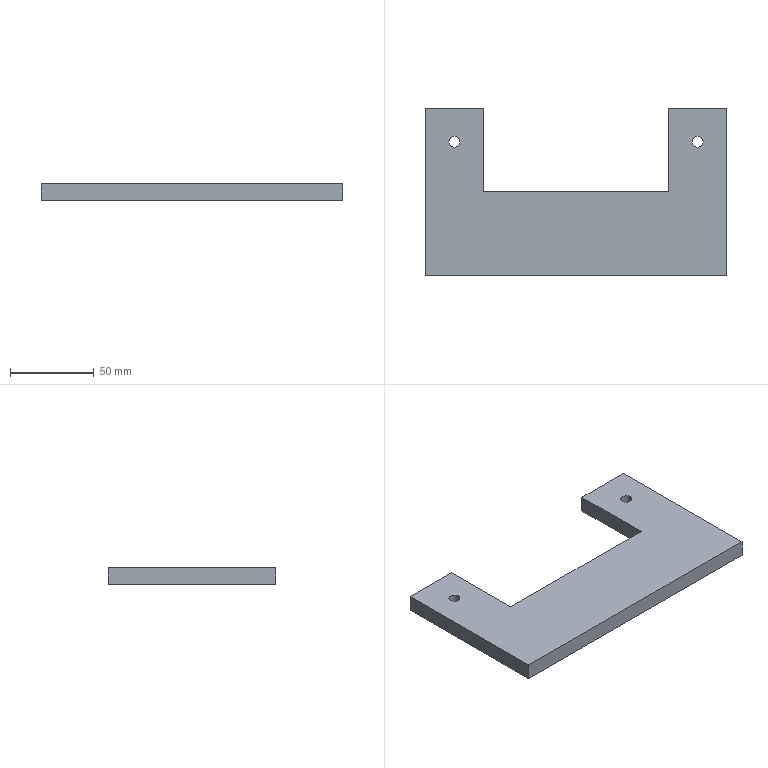Part | SolidWorks | features Extrusion 1, HoleWzd 1, ICE 1 | 1 solid | 14 faces | box 180 x 100 x 10 mm | volume 124316 mm3 | plane 10 | cylinder 4 | commonest cylinder face diameters 6.6 x4
STEP:
#1=CARTESIAN_POINT('',(69.2,30.,10.));
#2=VERTEX_POINT('',#1);
#3=CARTESIAN_POINT('',(75.8,30.,10.));
#4=VERTEX_POINT('',#3);
#5=CARTESIAN_POINT('',(72.5,30.,10.));
#6=DIRECTION('',(0.,0.,1.));
#7=DIRECTION('',(1.,0.,0.));
#8=AXIS2_PLACEMENT_3D('',#5,#6,#7);
#9=CIRCLE('',#8,3.3);
#10=EDGE_CURVE('',#2,#4,#9,.T.);
#11=ORIENTED_EDGE('',*,*,#10,.T.);
#12=CARTESIAN_POINT('',(75.8,30.,0.));
#13=VERTEX_POINT('',#12);
#14=CARTESIAN_POINT('',(75.8,30.,0.));
#15=DIRECTION('',(0.,0.,-1.));
#16=VECTOR('',#15,1000.);
#17=LINE('',#14,#16);
#18=EDGE_CURVE('',#4,#13,#17,.T.);
#19=ORIENTED_EDGE('',*,*,#18,.T.);
#20=CARTESIAN_POINT('',(69.2,30.,0.));
#21=VERTEX_POINT('',#20);
#22=CARTESIAN_POINT('',(72.5,30.,0.));
#23=DIRECTION('',(0.,0.,-1.));
#24=DIRECTION('',(-1.,0.,0.));
#25=AXIS2_PLACEMENT_3D('',#22,#23,#24);
#26=CIRCLE('',#25,3.3);
#27=EDGE_CURVE('',#13,#21,#26,.T.);
#28=ORIENTED_EDGE('',*,*,#27,.T.);
#29=CARTESIAN_POINT('',(69.2,30.,0.));
#30=DIRECTION('',(0.,0.,-1.));
#31=VECTOR('',#30,1000.);
#32=LINE('',#29,#31);
#33=EDGE_CURVE('',#2,#21,#32,.T.);
#34=ORIENTED_EDGE('',*,*,#33,.F.);
#35=EDGE_LOOP('',(#11,#19,#28,#34));
#36=FACE_OUTER_BOUND('',#35,.T.);
#37=CARTESIAN_POINT('',(72.5,30.,0.));
#38=DIRECTION('',(0.,0.,-1.));
#39=DIRECTION('',(-1.,0.,0.));
#40=AXIS2_PLACEMENT_3D('',#37,#38,#39);
#41=CYLINDRICAL_SURFACE('',#40,3.3);
#42=ADVANCED_FACE('',(#36),#41,.F.);
#43=CARTESIAN_POINT('',(-75.8,30.,10.));
#44=VERTEX_POINT('',#43);
#45=CARTESIAN_POINT('',(-69.2,30.,10.));
#46=VERTEX_POINT('',#45);
#47=CARTESIAN_POINT('',(-72.5,30.,10.));
#48=DIRECTION('',(0.,0.,1.));
#49=DIRECTION('',(1.,0.,0.));
#50=AXIS2_PLACEMENT_3D('',#47,#48,#49);
#51=CIRCLE('',#50,3.3);
#52=EDGE_CURVE('',#44,#46,#51,.T.);
#53=ORIENTED_EDGE('',*,*,#52,.T.);
#54=CARTESIAN_POINT('',(-69.2,30.,0.));
#55=VERTEX_POINT('',#54);
#56=CARTESIAN_POINT('',(-69.2,30.,0.));
#57=DIRECTION('',(0.,0.,-1.));
#58=VECTOR('',#57,1000.);
#59=LINE('',#56,#58);
#60=EDGE_CURVE('',#46,#55,#59,.T.);
#61=ORIENTED_EDGE('',*,*,#60,.T.);
#62=CARTESIAN_POINT('',(-75.8,30.,0.));
#63=VERTEX_POINT('',#62);
#64=CARTESIAN_POINT('',(-72.5,30.,0.));
#65=DIRECTION('',(0.,0.,-1.));
#66=DIRECTION('',(-1.,0.,0.));
#67=AXIS2_PLACEMENT_3D('',#64,#65,#66);
#68=CIRCLE('',#67,3.3);
#69=EDGE_CURVE('',#55,#63,#68,.T.);
#70=ORIENTED_EDGE('',*,*,#69,.T.);
#71=CARTESIAN_POINT('',(-75.8,30.,0.));
#72=DIRECTION('',(0.,0.,-1.));
#73=VECTOR('',#72,1000.);
#74=LINE('',#71,#73);
#75=EDGE_CURVE('',#44,#63,#74,.T.);
#76=ORIENTED_EDGE('',*,*,#75,.F.);
#77=EDGE_LOOP('',(#53,#61,#70,#76));
#78=FACE_OUTER_BOUND('',#77,.T.);
#79=CARTESIAN_POINT('',(-72.5,30.,0.));
#80=DIRECTION('',(0.,0.,-1.));
#81=DIRECTION('',(-1.,0.,0.));
#82=AXIS2_PLACEMENT_3D('',#79,#80,#81);
#83=CYLINDRICAL_SURFACE('',#82,3.3);
#84=ADVANCED_FACE('',(#78),#83,.F.);
#85=CARTESIAN_POINT('',(-55.,50.,0.));
#86=VERTEX_POINT('',#85);
#87=CARTESIAN_POINT('',(-90.,50.,0.));
#88=VERTEX_POINT('',#87);
#89=CARTESIAN_POINT('',(90.,50.,0.));
#90=DIRECTION('',(-1.,0.,0.));
#91=VECTOR('',#90,1000.);
#92=LINE('',#89,#91);
#93=EDGE_CURVE('',#86,#88,#92,.T.);
#94=ORIENTED_EDGE('',*,*,#93,.F.);
#95=CARTESIAN_POINT('',(-55.,0.,0.));
#96=VERTEX_POINT('',#95);
#97=CARTESIAN_POINT('',(-55.,100.,0.));
#98=DIRECTION('',(0.,1.,0.));
#99=VECTOR('',#98,1000.);
#100=LINE('',#97,#99);
#101=EDGE_CURVE('',#96,#86,#100,.T.);
#102=ORIENTED_EDGE('',*,*,#101,.F.);
#103=CARTESIAN_POINT('',(55.,0.,0.));
#104=VERTEX_POINT('',#103);
#105=CARTESIAN_POINT('',(55.,0.,0.));
#106=DIRECTION('',(-1.,0.,0.));
#107=VECTOR('',#106,1000.);
#108=LINE('',#105,#107);
#109=EDGE_CURVE('',#104,#96,#108,.T.);
#110=ORIENTED_EDGE('',*,*,#109,.F.);
#111=CARTESIAN_POINT('',(55.,50.,0.));
#112=VERTEX_POINT('',#111);
#113=CARTESIAN_POINT('',(55.,100.,0.));
#114=DIRECTION('',(0.,-1.,0.));
#115=VECTOR('',#114,1000.);
#116=LINE('',#113,#115);
#117=EDGE_CURVE('',#112,#104,#116,.T.);
#118=ORIENTED_EDGE('',*,*,#117,.F.);
#119=CARTESIAN_POINT('',(90.,50.,0.));
#120=VERTEX_POINT('',#119);
#121=CARTESIAN_POINT('',(90.,50.,0.));
#122=DIRECTION('',(-1.,0.,0.));
#123=VECTOR('',#122,1000.);
#124=LINE('',#121,#123);
#125=EDGE_CURVE('',#120,#112,#124,.T.);
#126=ORIENTED_EDGE('',*,*,#125,.F.);
#127=CARTESIAN_POINT('',(90.,-50.,0.));
#128=VERTEX_POINT('',#127);
#129=CARTESIAN_POINT('',(90.,-50.,0.));
#130=DIRECTION('',(0.,1.,0.));
#131=VECTOR('',#130,1000.);
#132=LINE('',#129,#131);
#133=EDGE_CURVE('',#128,#120,#132,.T.);
#134=ORIENTED_EDGE('',*,*,#133,.F.);
#135=CARTESIAN_POINT('',(-90.,-50.,0.));
#136=VERTEX_POINT('',#135);
#137=CARTESIAN_POINT('',(90.,-50.,0.));
#138=DIRECTION('',(1.,0.,0.));
#139=VECTOR('',#138,1000.);
#140=LINE('',#137,#139);
#141=EDGE_CURVE('',#136,#128,#140,.T.);
#142=ORIENTED_EDGE('',*,*,#141,.F.);
#143=CARTESIAN_POINT('',(-90.,-50.,0.));
#144=DIRECTION('',(0.,-1.,0.));
#145=VECTOR('',#144,1000.);
#146=LINE('',#143,#145);
#147=EDGE_CURVE('',#88,#136,#146,.T.);
#148=ORIENTED_EDGE('',*,*,#147,.F.);
#149=EDGE_LOOP('',(#94,#102,#110,#118,#126,#134,#142,#148));
#150=FACE_OUTER_BOUND('',#149,.T.);
#151=CARTESIAN_POINT('',(-72.5,30.,0.));
#152=DIRECTION('',(0.,0.,-1.));
#153=DIRECTION('',(-1.,0.,0.));
#154=AXIS2_PLACEMENT_3D('',#151,#152,#153);
#155=CIRCLE('',#154,3.3);
#156=EDGE_CURVE('',#63,#55,#155,.T.);
#157=ORIENTED_EDGE('',*,*,#156,.F.);
#158=ORIENTED_EDGE('',*,*,#69,.F.);
#159=EDGE_LOOP('',(#157,#158));
#160=FACE_BOUND('',#159,.T.);
#161=CARTESIAN_POINT('',(72.5,30.,0.));
#162=DIRECTION('',(0.,0.,-1.));
#163=DIRECTION('',(-1.,0.,0.));
#164=AXIS2_PLACEMENT_3D('',#161,#162,#163);
#165=CIRCLE('',#164,3.3);
#166=EDGE_CURVE('',#21,#13,#165,.T.);
#167=ORIENTED_EDGE('',*,*,#166,.F.);
#168=ORIENTED_EDGE('',*,*,#27,.F.);
#169=EDGE_LOOP('',(#167,#168));
#170=FACE_BOUND('',#169,.T.);
#171=CARTESIAN_POINT('',(0.,0.,0.));
#172=DIRECTION('',(0.,0.,1.));
#173=DIRECTION('',(1.,0.,0.));
#174=AXIS2_PLACEMENT_3D('',#171,#172,#173);
#175=PLANE('',#174);
#176=ADVANCED_FACE('',(#150,#160,#170),#175,.F.);
#177=CARTESIAN_POINT('',(-55.,50.,10.));
#178=VERTEX_POINT('',#177);
#179=CARTESIAN_POINT('',(-90.,50.,10.));
#180=VERTEX_POINT('',#179);
#181=CARTESIAN_POINT('',(90.,50.,10.));
#182=DIRECTION('',(-1.,0.,0.));
#183=VECTOR('',#182,1000.);
#184=LINE('',#181,#183);
#185=EDGE_CURVE('',#178,#180,#184,.T.);
#186=ORIENTED_EDGE('',*,*,#185,.F.);
#187=CARTESIAN_POINT('',(-55.,50.,-0.001));
#188=DIRECTION('',(0.,0.,1.));
#189=VECTOR('',#188,1000.);
#190=LINE('',#187,#189);
#191=EDGE_CURVE('',#86,#178,#190,.T.);
#192=ORIENTED_EDGE('',*,*,#191,.F.);
#193=ORIENTED_EDGE('',*,*,#93,.T.);
#194=CARTESIAN_POINT('',(-90.,50.,10.));
#195=DIRECTION('',(0.,0.,-1.));
#196=VECTOR('',#195,1000.);
#197=LINE('',#194,#196);
#198=EDGE_CURVE('',#180,#88,#197,.T.);
#199=ORIENTED_EDGE('',*,*,#198,.F.);
#200=EDGE_LOOP('',(#186,#192,#193,#199));
#201=FACE_OUTER_BOUND('',#200,.T.);
#202=CARTESIAN_POINT('',(90.,50.,10.));
#203=DIRECTION('',(0.,-1.,0.));
#204=DIRECTION('',(1.,0.,0.));
#205=AXIS2_PLACEMENT_3D('',#202,#203,#204);
#206=PLANE('',#205);
#207=ADVANCED_FACE('',(#201),#206,.F.);
#208=ORIENTED_EDGE('',*,*,#147,.T.);
#209=CARTESIAN_POINT('',(-90.,-50.,10.));
#210=VERTEX_POINT('',#209);
#211=CARTESIAN_POINT('',(-90.,-50.,10.));
#212=DIRECTION('',(0.,0.,-1.));
#213=VECTOR('',#212,1000.);
#214=LINE('',#211,#213);
#215=EDGE_CURVE('',#210,#136,#214,.T.);
#216=ORIENTED_EDGE('',*,*,#215,.F.);
#217=CARTESIAN_POINT('',(-90.,-50.,10.));
#218=DIRECTION('',(0.,-1.,0.));
#219=VECTOR('',#218,1000.);
#220=LINE('',#217,#219);
#221=EDGE_CURVE('',#180,#210,#220,.T.);
#222=ORIENTED_EDGE('',*,*,#221,.F.);
#223=ORIENTED_EDGE('',*,*,#198,.T.);
#224=EDGE_LOOP('',(#208,#216,#222,#223));
#225=FACE_OUTER_BOUND('',#224,.T.);
#226=CARTESIAN_POINT('',(-90.,-50.,10.));
#227=DIRECTION('',(1.,0.,0.));
#228=DIRECTION('',(0.,0.,-1.));
#229=AXIS2_PLACEMENT_3D('',#226,#227,#228);
#230=PLANE('',#229);
#231=ADVANCED_FACE('',(#225),#230,.F.);
#232=ORIENTED_EDGE('',*,*,#141,.T.);
#233=CARTESIAN_POINT('',(90.,-50.,10.));
#234=VERTEX_POINT('',#233);
#235=CARTESIAN_POINT('',(90.,-50.,10.));
#236=DIRECTION('',(0.,0.,-1.));
#237=VECTOR('',#236,1000.);
#238=LINE('',#235,#237);
#239=EDGE_CURVE('',#234,#128,#238,.T.);
#240=ORIENTED_EDGE('',*,*,#239,.F.);
#241=CARTESIAN_POINT('',(90.,-50.,10.));
#242=DIRECTION('',(1.,0.,0.));
#243=VECTOR('',#242,1000.);
#244=LINE('',#241,#243);
#245=EDGE_CURVE('',#210,#234,#244,.T.);
#246=ORIENTED_EDGE('',*,*,#245,.F.);
#247=ORIENTED_EDGE('',*,*,#215,.T.);
#248=EDGE_LOOP('',(#232,#240,#246,#247));
#249=FACE_OUTER_BOUND('',#248,.T.);
#250=CARTESIAN_POINT('',(90.,-50.,10.));
#251=DIRECTION('',(0.,1.,0.));
#252=DIRECTION('',(-1.,0.,0.));
#253=AXIS2_PLACEMENT_3D('',#250,#251,#252);
#254=PLANE('',#253);
#255=ADVANCED_FACE('',(#249),#254,.F.);
#256=ORIENTED_EDGE('',*,*,#133,.T.);
#257=CARTESIAN_POINT('',(90.,50.,10.));
#258=VERTEX_POINT('',#257);
#259=CARTESIAN_POINT('',(90.,50.,10.));
#260=DIRECTION('',(0.,0.,-1.));
#261=VECTOR('',#260,1000.);
#262=LINE('',#259,#261);
#263=EDGE_CURVE('',#258,#120,#262,.T.);
#264=ORIENTED_EDGE('',*,*,#263,.F.);
#265=CARTESIAN_POINT('',(90.,-50.,10.));
#266=DIRECTION('',(0.,1.,0.));
#267=VECTOR('',#266,1000.);
#268=LINE('',#265,#267);
#269=EDGE_CURVE('',#234,#258,#268,.T.);
#270=ORIENTED_EDGE('',*,*,#269,.F.);
#271=ORIENTED_EDGE('',*,*,#239,.T.);
#272=EDGE_LOOP('',(#256,#264,#270,#271));
#273=FACE_OUTER_BOUND('',#272,.T.);
#274=CARTESIAN_POINT('',(90.,-50.,10.));
#275=DIRECTION('',(-1.,0.,0.));
#276=DIRECTION('',(0.,0.,1.));
#277=AXIS2_PLACEMENT_3D('',#274,#275,#276);
#278=PLANE('',#277);
#279=ADVANCED_FACE('',(#273),#278,.F.);
#280=ORIENTED_EDGE('',*,*,#125,.T.);
#281=CARTESIAN_POINT('',(55.,50.,10.));
#282=VERTEX_POINT('',#281);
#283=CARTESIAN_POINT('',(55.,50.,-0.001));
#284=DIRECTION('',(0.,0.,-1.));
#285=VECTOR('',#284,1000.);
#286=LINE('',#283,#285);
#287=EDGE_CURVE('',#282,#112,#286,.T.);
#288=ORIENTED_EDGE('',*,*,#287,.F.);
#289=CARTESIAN_POINT('',(90.,50.,10.));
#290=DIRECTION('',(-1.,0.,0.));
#291=VECTOR('',#290,1000.);
#292=LINE('',#289,#291);
#293=EDGE_CURVE('',#258,#282,#292,.T.);
#294=ORIENTED_EDGE('',*,*,#293,.F.);
#295=ORIENTED_EDGE('',*,*,#263,.T.);
#296=EDGE_LOOP('',(#280,#288,#294,#295));
#297=FACE_OUTER_BOUND('',#296,.T.);
#298=CARTESIAN_POINT('',(90.,50.,10.));
#299=DIRECTION('',(0.,-1.,0.));
#300=DIRECTION('',(1.,0.,0.));
#301=AXIS2_PLACEMENT_3D('',#298,#299,#300);
#302=PLANE('',#301);
#303=ADVANCED_FACE('',(#297),#302,.F.);
#304=ORIENTED_EDGE('',*,*,#10,.F.);
#305=CARTESIAN_POINT('',(72.5,30.,10.));
#306=DIRECTION('',(0.,0.,1.));
#307=DIRECTION('',(1.,0.,0.));
#308=AXIS2_PLACEMENT_3D('',#305,#306,#307);
#309=CIRCLE('',#308,3.3);
#310=EDGE_CURVE('',#4,#2,#309,.T.);
#311=ORIENTED_EDGE('',*,*,#310,.F.);
#312=EDGE_LOOP('',(#304,#311));
#313=FACE_BOUND('',#312,.T.);
#314=ORIENTED_EDGE('',*,*,#52,.F.);
#315=CARTESIAN_POINT('',(-72.5,30.,10.));
#316=DIRECTION('',(0.,0.,1.));
#317=DIRECTION('',(1.,0.,0.));
#318=AXIS2_PLACEMENT_3D('',#315,#316,#317);
#319=CIRCLE('',#318,3.3);
#320=EDGE_CURVE('',#46,#44,#319,.T.);
#321=ORIENTED_EDGE('',*,*,#320,.F.);
#322=EDGE_LOOP('',(#314,#321));
#323=FACE_BOUND('',#322,.T.);
#324=CARTESIAN_POINT('',(-55.,0.,10.));
#325=VERTEX_POINT('',#324);
#326=CARTESIAN_POINT('',(-55.,100.,10.));
#327=DIRECTION('',(0.,-1.,0.));
#328=VECTOR('',#327,1000.);
#329=LINE('',#326,#328);
#330=EDGE_CURVE('',#178,#325,#329,.T.);
#331=ORIENTED_EDGE('',*,*,#330,.F.);
#332=ORIENTED_EDGE('',*,*,#185,.T.);
#333=ORIENTED_EDGE('',*,*,#221,.T.);
#334=ORIENTED_EDGE('',*,*,#245,.T.);
#335=ORIENTED_EDGE('',*,*,#269,.T.);
#336=ORIENTED_EDGE('',*,*,#293,.T.);
#337=CARTESIAN_POINT('',(55.,0.,10.));
#338=VERTEX_POINT('',#337);
#339=CARTESIAN_POINT('',(55.,100.,10.));
#340=DIRECTION('',(0.,1.,0.));
#341=VECTOR('',#340,1000.);
#342=LINE('',#339,#341);
#343=EDGE_CURVE('',#338,#282,#342,.T.);
#344=ORIENTED_EDGE('',*,*,#343,.F.);
#345=CARTESIAN_POINT('',(55.,0.,10.));
#346=DIRECTION('',(1.,0.,0.));
#347=VECTOR('',#346,1000.);
#348=LINE('',#345,#347);
#349=EDGE_CURVE('',#325,#338,#348,.T.);
#350=ORIENTED_EDGE('',*,*,#349,.F.);
#351=EDGE_LOOP('',(#331,#332,#333,#334,#335,#336,#344,#350));
#352=FACE_OUTER_BOUND('',#351,.T.);
#353=CARTESIAN_POINT('',(0.,0.,10.));
#354=DIRECTION('',(0.,0.,1.));
#355=DIRECTION('',(1.,0.,0.));
#356=AXIS2_PLACEMENT_3D('',#353,#354,#355);
#357=PLANE('',#356);
#358=ADVANCED_FACE('',(#313,#323,#352),#357,.T.);
#359=ORIENTED_EDGE('',*,*,#191,.T.);
#360=ORIENTED_EDGE('',*,*,#330,.T.);
#361=CARTESIAN_POINT('',(-55.,0.,-0.001));
#362=DIRECTION('',(0.,0.,1.));
#363=VECTOR('',#362,1000.);
#364=LINE('',#361,#363);
#365=EDGE_CURVE('',#96,#325,#364,.T.);
#366=ORIENTED_EDGE('',*,*,#365,.F.);
#367=ORIENTED_EDGE('',*,*,#101,.T.);
#368=EDGE_LOOP('',(#359,#360,#366,#367));
#369=FACE_OUTER_BOUND('',#368,.T.);
#370=CARTESIAN_POINT('',(-55.,100.,-0.001));
#371=DIRECTION('',(-1.,0.,0.));
#372=DIRECTION('',(0.,0.,1.));
#373=AXIS2_PLACEMENT_3D('',#370,#371,#372);
#374=PLANE('',#373);
#375=ADVANCED_FACE('',(#369),#374,.F.);
#376=ORIENTED_EDGE('',*,*,#287,.T.);
#377=ORIENTED_EDGE('',*,*,#117,.T.);
#378=CARTESIAN_POINT('',(55.,0.,-0.001));
#379=DIRECTION('',(0.,0.,1.));
#380=VECTOR('',#379,1000.);
#381=LINE('',#378,#380);
#382=EDGE_CURVE('',#104,#338,#381,.T.);
#383=ORIENTED_EDGE('',*,*,#382,.T.);
#384=ORIENTED_EDGE('',*,*,#343,.T.);
#385=EDGE_LOOP('',(#376,#377,#383,#384));
#386=FACE_OUTER_BOUND('',#385,.T.);
#387=CARTESIAN_POINT('',(55.,100.,-0.001));
#388=DIRECTION('',(1.,0.,0.));
#389=DIRECTION('',(0.,0.,-1.));
#390=AXIS2_PLACEMENT_3D('',#387,#388,#389);
#391=PLANE('',#390);
#392=ADVANCED_FACE('',(#386),#391,.F.);
#393=ORIENTED_EDGE('',*,*,#109,.T.);
#394=ORIENTED_EDGE('',*,*,#365,.T.);
#395=ORIENTED_EDGE('',*,*,#349,.T.);
#396=ORIENTED_EDGE('',*,*,#382,.F.);
#397=EDGE_LOOP('',(#393,#394,#395,#396));
#398=FACE_OUTER_BOUND('',#397,.T.);
#399=CARTESIAN_POINT('',(55.,0.,-0.001));
#400=DIRECTION('',(0.,-1.,0.));
#401=DIRECTION('',(1.,0.,0.));
#402=AXIS2_PLACEMENT_3D('',#399,#400,#401);
#403=PLANE('',#402);
#404=ADVANCED_FACE('',(#398),#403,.F.);
#405=ORIENTED_EDGE('',*,*,#60,.F.);
#406=ORIENTED_EDGE('',*,*,#320,.T.);
#407=ORIENTED_EDGE('',*,*,#75,.T.);
#408=ORIENTED_EDGE('',*,*,#156,.T.);
#409=EDGE_LOOP('',(#405,#406,#407,#408));
#410=FACE_OUTER_BOUND('',#409,.T.);
#411=CARTESIAN_POINT('',(-72.5,30.,0.));
#412=DIRECTION('',(0.,0.,-1.));
#413=DIRECTION('',(-1.,0.,0.));
#414=AXIS2_PLACEMENT_3D('',#411,#412,#413);
#415=CYLINDRICAL_SURFACE('',#414,3.3);
#416=ADVANCED_FACE('',(#410),#415,.F.);
#417=ORIENTED_EDGE('',*,*,#18,.F.);
#418=ORIENTED_EDGE('',*,*,#310,.T.);
#419=ORIENTED_EDGE('',*,*,#33,.T.);
#420=ORIENTED_EDGE('',*,*,#166,.T.);
#421=EDGE_LOOP('',(#417,#418,#419,#420));
#422=FACE_OUTER_BOUND('',#421,.T.);
#423=CARTESIAN_POINT('',(72.5,30.,0.));
#424=DIRECTION('',(0.,0.,-1.));
#425=DIRECTION('',(-1.,0.,0.));
#426=AXIS2_PLACEMENT_3D('',#423,#424,#425);
#427=CYLINDRICAL_SURFACE('',#426,3.3);
#428=ADVANCED_FACE('',(#422),#427,.F.);
#429=CLOSED_SHELL('',(#42,#84,#176,#207,#231,#255,#279,#303,#358,#375,#392,#404,#416,#428));
#430=MANIFOLD_SOLID_BREP('',#429);
#431=CARTESIAN_POINT('',(0.,0.,0.));
#432=DIRECTION('',(0.,0.,1.));
#433=DIRECTION('',(1.,0.,0.));
#434=AXIS2_PLACEMENT_3D('',#431,#432,#433);
#435=(LENGTH_UNIT()NAMED_UNIT(*)SI_UNIT(.MILLI.,.METRE.));
#436=UNCERTAINTY_MEASURE_WITH_UNIT(LENGTH_MEASURE(0.00001),#435,'','');
#437=(NAMED_UNIT(*)PLANE_ANGLE_UNIT()SI_UNIT($,.RADIAN.));
#438=(NAMED_UNIT(*)SI_UNIT($,.STERADIAN.)SOLID_ANGLE_UNIT());
#439=(GEOMETRIC_REPRESENTATION_CONTEXT(3)GLOBAL_UNCERTAINTY_ASSIGNED_CONTEXT((#436))GLOBAL_UNIT_ASSIGNED_CONTEXT((#435,#437,#438))REPRESENTATION_CONTEXT('',''));
#440=ADVANCED_BREP_SHAPE_REPRESENTATION('',(#430,#434),#439);